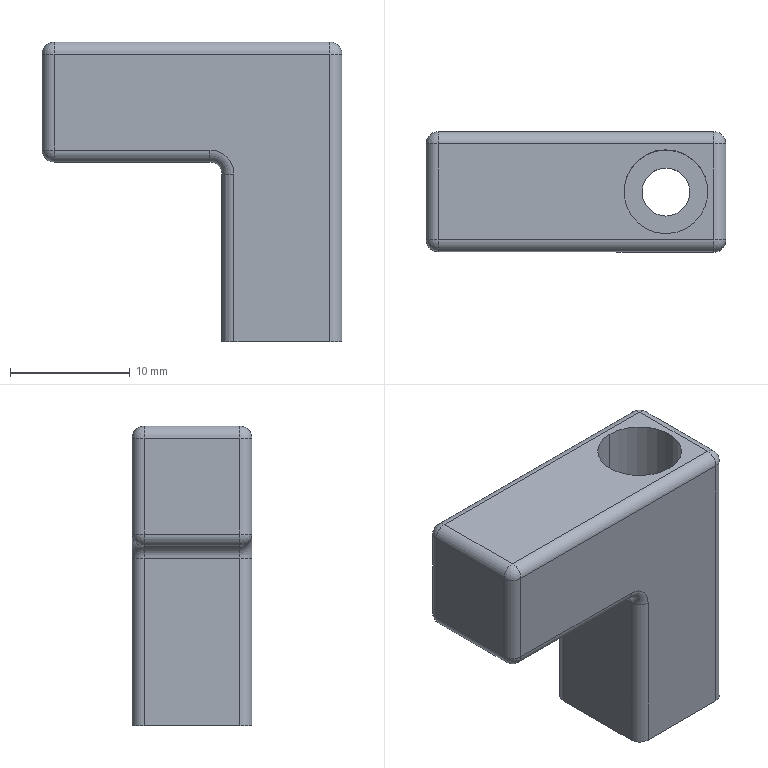NC program | NX | posted with a generic post | part box 25 x 10 x 25 mm
Lines 1 to 1607 of 2000, first 1374 of 1599 lines:
N10 G17 G21 G94 G90
(FLOOR_WALL , TOOL : D63)
N12 T01 M6
N14 G54
N16 G17 G0 G90 X-50. Y0. S6500 M3
N18 G43 Z13. H1
N20 Z3.
N22 G94 G1 Z0. F1250.
N24 X-47.
N26 X47.
N28 X50.
N30 Z3.
N32 G0 Z13.
N34 M5
(ZLEVEL_PROFILE , TOOL : D10)
N36 T09 M6
N38 G54
N40 G17 G0 G90 X2.496 Y10.099 S9500 M3
N42 G43 Z11. H9
N44 Z1.5
N46 G94 G1 X11.5 Z1.028 F1000.
N48 X12.106 Z0.996
N50 X13.737 Y9.707 Z0.908
N52 X15.2 Y8.886 Z0.821
N54 X16.386 Y7.7 Z0.733
N56 X17.206 Y6.237 Z0.645
N58 X17.599 Y4.606 Z0.557
N60 Y4. Z0.525
N62 Y-4. Z0.106
N64 Y-4.606 Z0.074
N66 X17.206 Y-6.237 Z-0.014
N68 X16.386 Y-7.7 Z-0.102
N70 X15.2 Y-8.886 Z-0.19
N72 X13.737 Y-9.707 Z-0.278
N74 X12.106 Y-10.099 Z-0.366
N76 X11.5 Z-0.397
N78 X0. Z-1.
N80 X-11.5 F3000.
N82 G2 X-17.594 Y-4.223 R6.098
N84 G1 X-17.599 Y-4.
N86 Y4.
N88 G2 X-11.5 Y10.099 R6.099
N90 G1 X11.5
N92 G2 X17.599 Y4. R6.099
N94 G1 Y-4.
N96 G2 X11.5 Y-10.099 R6.099
N98 G1 X0.
N100 X-0.387 Y-10.1 Z-1.007
N102 X-10.839 Z-1.189
N104 X-11.226 Z-1.196
N106 X-11.613 Y-10.099 Z-1.203
N108 X-11.999 Y-10.08 Z-1.209
N110 X-12.384 Y-10.036 Z-1.216
N112 X-12.765 Y-9.967 Z-1.223
N114 X-13.141 Y-9.875 Z-1.23
N116 X-13.51 Y-9.759 Z-1.236
N118 X-13.871 Y-9.62 Z-1.243
N120 X-14.223 Y-9.458 Z-1.25
N122 X-14.564 Y-9.275 Z-1.257
N124 X-14.892 Y-9.07 Z-1.264
N126 X-15.207 Y-8.844 Z-1.27
N128 X-15.507 Y-8.6 Z-1.277
N130 X-15.79 Y-8.336 Z-1.284
N132 X-16.057 Y-8.055 Z-1.291
N134 X-16.305 Y-7.758 Z-1.297
N136 X-16.533 Y-7.446 Z-1.304
N138 X-16.742 Y-7.12 Z-1.311
N140 X-16.929 Y-6.781 Z-1.318
N142 X-17.095 Y-6.431 Z-1.324
N144 X-17.238 Y-6.071 Z-1.331
N146 X-17.357 Y-5.703 Z-1.338
N148 X-17.454 Y-5.328 Z-1.345
N150 X-17.526 Y-4.948 Z-1.351
N152 X-17.574 Y-4.564 Z-1.358
N154 X-17.597 Y-4.177 Z-1.365
N156 X-17.6 Y-3.79 Z-1.372
N158 Y-3.403 Z-1.378
N160 Y3.565 Z-1.5
N162 Y3.952 Z-1.507
N164 X-17.591 Y4.339 Z-1.514
N166 X-17.557 Y4.724 Z-1.52
N168 X-17.499 Y5.107 Z-1.527
N170 X-17.416 Y5.485 Z-1.534
N172 X-17.31 Y5.857 Z-1.541
N174 X-17.181 Y6.222 Z-1.547
N176 X-17.028 Y6.578 Z-1.554
N178 X-16.854 Y6.924 Z-1.561
N180 X-16.658 Y7.257 Z-1.568
N182 X-16.441 Y7.578 Z-1.574
N184 X-16.204 Y7.884 Z-1.581
N186 X-15.948 Y8.174 Z-1.588
N188 X-15.674 Y8.448 Z-1.595
N190 X-15.384 Y8.704 Z-1.601
N192 X-15.078 Y8.941 Z-1.608
N194 X-14.757 Y9.158 Z-1.615
N196 X-14.423 Y9.354 Z-1.622
N198 X-14.078 Y9.529 Z-1.628
N200 X-13.722 Y9.681 Z-1.635
N202 X-13.357 Y9.81 Z-1.642
N204 X-12.985 Y9.916 Z-1.649
N206 X-12.607 Y9.999 Z-1.655
N208 X-12.224 Y10.057 Z-1.662
N210 X-11.838 Y10.091 Z-1.669
N212 X-11.451 Y10.1 Z-1.676
N214 X7.129 Z-2.
N216 X11.5
N218 G2 X17.6 Y4. R6.1
N220 G1 Y-4.
N222 G2 X11.5 Y-10.1 R6.1
N224 G1 X0.
N226 X-10.839 Z-2.189
N228 X-11.226 Z-2.196
N230 X-11.613 Y-10.099 Z-2.203
N232 X-11.999 Y-10.08 Z-2.209
N234 X-12.384 Y-10.036 Z-2.216
N236 X-12.765 Y-9.967 Z-2.223
N238 X-13.141 Y-9.875 Z-2.23
N240 X-13.51 Y-9.759 Z-2.236
N242 X-13.871 Y-9.62 Z-2.243
N244 X-14.223 Y-9.459 Z-2.25
N246 X-14.564 Y-9.275 Z-2.257
N248 X-14.892 Y-9.07 Z-2.264
N250 X-15.207 Y-8.845 Z-2.27
N252 X-15.506 Y-8.6 Z-2.277
N254 X-15.79 Y-8.337 Z-2.284
N256 X-16.056 Y-8.056 Z-2.291
N258 X-16.304 Y-7.759 Z-2.297
N260 X-16.533 Y-7.446 Z-2.304
N262 X-16.742 Y-7.12 Z-2.311
N264 X-16.929 Y-6.782 Z-2.318
N266 X-17.094 Y-6.432 Z-2.324
N268 X-17.237 Y-6.072 Z-2.331
N270 X-17.357 Y-5.704 Z-2.338
N272 X-17.453 Y-5.329 Z-2.345
N274 X-17.526 Y-4.949 Z-2.351
N276 X-17.574 Y-4.565 Z-2.358
N278 X-17.597 Y-4.179 Z-2.365
N280 X-17.6 Y-3.792 Z-2.372
N282 Y-3.405 Z-2.378
N284 Y3.563 Z-2.5
N286 Y3.95 Z-2.507
N288 X-17.591 Y4.337 Z-2.514
N290 X-17.557 Y4.723 Z-2.52
N292 X-17.499 Y5.105 Z-2.527
N294 X-17.417 Y5.484 Z-2.534
N296 X-17.311 Y5.856 Z-2.541
N298 X-17.181 Y6.221 Z-2.547
N300 X-17.029 Y6.576 Z-2.554
N302 X-16.855 Y6.922 Z-2.561
N304 X-16.659 Y7.256 Z-2.568
N306 X-16.442 Y7.576 Z-2.574
N308 X-16.205 Y7.882 Z-2.581
N310 X-15.949 Y8.173 Z-2.588
N312 X-15.676 Y8.447 Z-2.595
N314 X-15.385 Y8.702 Z-2.601
N316 X-15.079 Y8.939 Z-2.608
N318 X-14.759 Y9.156 Z-2.615
N320 X-14.425 Y9.353 Z-2.622
N322 X-14.08 Y9.527 Z-2.628
N324 X-13.724 Y9.68 Z-2.635
N326 X-13.36 Y9.81 Z-2.642
N328 X-12.988 Y9.916 Z-2.649
N330 X-12.609 Y9.998 Z-2.655
N332 X-12.227 Y10.057 Z-2.662
N334 X-11.841 Y10.09 Z-2.669
N336 X-11.454 Y10.1 Z-2.676
N338 X7.126 Z-3.
N340 X11.5
N342 G2 X17.6 Y4. R6.1
N344 G1 Y-4.
N346 G2 X11.5 Y-10.1 R6.1
N348 G1 X0.
N350 X-10.839 Z-3.189
N352 X-11.226 Z-3.196
N354 X-11.613 Y-10.099 Z-3.203
N356 X-11.999 Y-10.08 Z-3.209
N358 X-12.384 Y-10.036 Z-3.216
N360 X-12.765 Y-9.967 Z-3.223
N362 X-13.141 Y-9.875 Z-3.23
N364 X-13.51 Y-9.759 Z-3.236
N366 X-13.871 Y-9.62 Z-3.243
N368 X-14.223 Y-9.459 Z-3.25
N370 X-14.564 Y-9.275 Z-3.257
N372 X-14.892 Y-9.07 Z-3.264
N374 X-15.207 Y-8.845 Z-3.27
N376 X-15.506 Y-8.6 Z-3.277
N378 X-15.79 Y-8.337 Z-3.284
N380 X-16.056 Y-8.056 Z-3.291
N382 X-16.304 Y-7.759 Z-3.297
N384 X-16.533 Y-7.446 Z-3.304
N386 X-16.742 Y-7.12 Z-3.311
N388 X-16.929 Y-6.782 Z-3.318
N390 X-17.094 Y-6.432 Z-3.324
N392 X-17.237 Y-6.072 Z-3.331
N394 X-17.357 Y-5.704 Z-3.338
N396 X-17.453 Y-5.329 Z-3.345
N398 X-17.526 Y-4.949 Z-3.351
N400 X-17.574 Y-4.565 Z-3.358
N402 X-17.597 Y-4.179 Z-3.365
N404 X-17.6 Y-3.792 Z-3.372
N406 Y-3.405 Z-3.378
N408 Y3.563 Z-3.5
N410 Y3.95 Z-3.507
N412 X-17.591 Y4.337 Z-3.514
N414 X-17.557 Y4.723 Z-3.52
N416 X-17.499 Y5.105 Z-3.527
N418 X-17.417 Y5.484 Z-3.534
N420 X-17.311 Y5.856 Z-3.541
N422 X-17.181 Y6.221 Z-3.547
N424 X-17.029 Y6.576 Z-3.554
N426 X-16.855 Y6.922 Z-3.561
N428 X-16.659 Y7.256 Z-3.568
N430 X-16.442 Y7.576 Z-3.574
N432 X-16.205 Y7.882 Z-3.581
N434 X-15.949 Y8.173 Z-3.588
N436 X-15.676 Y8.447 Z-3.595
N438 X-15.385 Y8.702 Z-3.601
N440 X-15.079 Y8.939 Z-3.608
N442 X-14.759 Y9.156 Z-3.615
N444 X-14.425 Y9.353 Z-3.622
N446 X-14.08 Y9.527 Z-3.628
N448 X-13.724 Y9.68 Z-3.635
N450 X-13.36 Y9.81 Z-3.642
N452 X-12.988 Y9.916 Z-3.649
N454 X-12.609 Y9.998 Z-3.655
N456 X-12.227 Y10.057 Z-3.662
N458 X-11.841 Y10.09 Z-3.669
N460 X-11.454 Y10.1 Z-3.676
N462 X7.126 Z-4.
N464 X11.5
N466 G2 X17.6 Y4. R6.1
N468 G1 Y-4.
N470 G2 X11.5 Y-10.1 R6.1
N472 G1 X0.
N474 X-10.839 Z-4.189
N476 X-11.226 Z-4.196
N478 X-11.613 Y-10.099 Z-4.203
N480 X-11.999 Y-10.08 Z-4.209
N482 X-12.384 Y-10.036 Z-4.216
N484 X-12.765 Y-9.967 Z-4.223
N486 X-13.141 Y-9.875 Z-4.23
N488 X-13.51 Y-9.759 Z-4.236
N490 X-13.871 Y-9.62 Z-4.243
N492 X-14.223 Y-9.459 Z-4.25
N494 X-14.564 Y-9.275 Z-4.257
N496 X-14.892 Y-9.07 Z-4.264
N498 X-15.207 Y-8.845 Z-4.27
N500 X-15.506 Y-8.6 Z-4.277
N502 X-15.79 Y-8.337 Z-4.284
N504 X-16.056 Y-8.056 Z-4.291
N506 X-16.304 Y-7.759 Z-4.297
N508 X-16.533 Y-7.446 Z-4.304
N510 X-16.742 Y-7.12 Z-4.311
N512 X-16.929 Y-6.782 Z-4.318
N514 X-17.094 Y-6.432 Z-4.324
N516 X-17.237 Y-6.072 Z-4.331
N518 X-17.357 Y-5.704 Z-4.338
N520 X-17.453 Y-5.329 Z-4.345
N522 X-17.526 Y-4.949 Z-4.351
N524 X-17.574 Y-4.565 Z-4.358
N526 X-17.597 Y-4.179 Z-4.365
N528 X-17.6 Y-3.792 Z-4.372
N530 Y-3.405 Z-4.378
N532 Y3.563 Z-4.5
N534 Y3.95 Z-4.507
N536 X-17.591 Y4.337 Z-4.514
N538 X-17.557 Y4.723 Z-4.52
N540 X-17.499 Y5.105 Z-4.527
N542 X-17.417 Y5.484 Z-4.534
N544 X-17.311 Y5.856 Z-4.541
N546 X-17.181 Y6.221 Z-4.547
N548 X-17.029 Y6.576 Z-4.554
N550 X-16.855 Y6.922 Z-4.561
N552 X-16.659 Y7.256 Z-4.568
N554 X-16.442 Y7.576 Z-4.574
N556 X-16.205 Y7.882 Z-4.581
N558 X-15.949 Y8.173 Z-4.588
N560 X-15.676 Y8.447 Z-4.595
N562 X-15.385 Y8.702 Z-4.601
N564 X-15.079 Y8.939 Z-4.608
N566 X-14.759 Y9.156 Z-4.615
N568 X-14.425 Y9.353 Z-4.622
N570 X-14.08 Y9.527 Z-4.628
N572 X-13.724 Y9.68 Z-4.635
N574 X-13.36 Y9.81 Z-4.642
N576 X-12.988 Y9.916 Z-4.649
N578 X-12.609 Y9.998 Z-4.655
N580 X-12.227 Y10.057 Z-4.662
N582 X-11.841 Y10.09 Z-4.669
N584 X-11.454 Y10.1 Z-4.676
N586 X7.126 Z-5.
N588 X11.5
N590 G2 X17.6 Y4. R6.1
N592 G1 Y-4.
N594 G2 X11.5 Y-10.1 R6.1
N596 G1 X0.
N598 X-10.839 Z-5.189
N600 X-11.226 Z-5.196
N602 X-11.613 Y-10.099 Z-5.203
N604 X-11.999 Y-10.08 Z-5.209
N606 X-12.384 Y-10.036 Z-5.216
N608 X-12.765 Y-9.967 Z-5.223
N610 X-13.141 Y-9.875 Z-5.23
N612 X-13.51 Y-9.759 Z-5.236
N614 X-13.871 Y-9.62 Z-5.243
N616 X-14.223 Y-9.459 Z-5.25
N618 X-14.564 Y-9.275 Z-5.257
N620 X-14.892 Y-9.07 Z-5.264
N622 X-15.207 Y-8.845 Z-5.27
N624 X-15.506 Y-8.6 Z-5.277
N626 X-15.79 Y-8.337 Z-5.284
N628 X-16.056 Y-8.056 Z-5.291
N630 X-16.304 Y-7.759 Z-5.297
N632 X-16.533 Y-7.446 Z-5.304
N634 X-16.742 Y-7.12 Z-5.311
N636 X-16.929 Y-6.782 Z-5.318
N638 X-17.094 Y-6.432 Z-5.324
N640 X-17.237 Y-6.072 Z-5.331
N642 X-17.357 Y-5.704 Z-5.338
N644 X-17.453 Y-5.329 Z-5.345
N646 X-17.526 Y-4.949 Z-5.351
N648 X-17.574 Y-4.565 Z-5.358
N650 X-17.597 Y-4.179 Z-5.365
N652 X-17.6 Y-3.792 Z-5.372
N654 Y-3.405 Z-5.378
N656 Y3.563 Z-5.5
N658 Y3.95 Z-5.507
N660 X-17.591 Y4.337 Z-5.514
N662 X-17.557 Y4.723 Z-5.52
N664 X-17.499 Y5.105 Z-5.527
N666 X-17.417 Y5.484 Z-5.534
N668 X-17.311 Y5.856 Z-5.541
N670 X-17.181 Y6.221 Z-5.547
N672 X-17.029 Y6.576 Z-5.554
N674 X-16.855 Y6.922 Z-5.561
N676 X-16.659 Y7.256 Z-5.568
N678 X-16.442 Y7.576 Z-5.574
N680 X-16.205 Y7.882 Z-5.581
N682 X-15.949 Y8.173 Z-5.588
N684 X-15.676 Y8.447 Z-5.595
N686 X-15.385 Y8.702 Z-5.601
N688 X-15.079 Y8.939 Z-5.608
N690 X-14.759 Y9.156 Z-5.615
N692 X-14.425 Y9.353 Z-5.622
N694 X-14.08 Y9.527 Z-5.628
N696 X-13.724 Y9.68 Z-5.635
N698 X-13.36 Y9.81 Z-5.642
N700 X-12.988 Y9.916 Z-5.649
N702 X-12.609 Y9.998 Z-5.655
N704 X-12.227 Y10.057 Z-5.662
N706 X-11.841 Y10.09 Z-5.669
N708 X-11.454 Y10.1 Z-5.676
N710 X7.126 Z-6.
N712 X11.5
N714 G2 X17.6 Y4. R6.1
N716 G1 Y-4.
N718 G2 X11.5 Y-10.1 R6.1
N720 G1 X0.
N722 X-10.839 Z-6.189
N724 X-11.226 Z-6.196
N726 X-11.613 Y-10.099 Z-6.203
N728 X-11.999 Y-10.08 Z-6.209
N730 X-12.384 Y-10.036 Z-6.216
N732 X-12.765 Y-9.967 Z-6.223
N734 X-13.141 Y-9.875 Z-6.23
N736 X-13.51 Y-9.759 Z-6.236
N738 X-13.871 Y-9.62 Z-6.243
N740 X-14.223 Y-9.459 Z-6.25
N742 X-14.564 Y-9.275 Z-6.257
N744 X-14.892 Y-9.07 Z-6.264
N746 X-15.207 Y-8.845 Z-6.27
N748 X-15.506 Y-8.6 Z-6.277
N750 X-15.79 Y-8.337 Z-6.284
N752 X-16.056 Y-8.056 Z-6.291
N754 X-16.304 Y-7.759 Z-6.297
N756 X-16.533 Y-7.446 Z-6.304
N758 X-16.742 Y-7.12 Z-6.311
N760 X-16.929 Y-6.782 Z-6.318
N762 X-17.094 Y-6.432 Z-6.324
N764 X-17.237 Y-6.072 Z-6.331
N766 X-17.357 Y-5.704 Z-6.338
N768 X-17.453 Y-5.329 Z-6.345
N770 X-17.526 Y-4.949 Z-6.351
N772 X-17.574 Y-4.565 Z-6.358
N774 X-17.597 Y-4.179 Z-6.365
N776 X-17.6 Y-3.792 Z-6.372
N778 Y-3.405 Z-6.378
N780 Y3.563 Z-6.5
N782 Y3.95 Z-6.507
N784 X-17.591 Y4.337 Z-6.514
N786 X-17.557 Y4.723 Z-6.52
N788 X-17.499 Y5.105 Z-6.527
N790 X-17.417 Y5.484 Z-6.534
N792 X-17.311 Y5.856 Z-6.541
N794 X-17.181 Y6.221 Z-6.547
N796 X-17.029 Y6.576 Z-6.554
N798 X-16.855 Y6.922 Z-6.561
N800 X-16.659 Y7.256 Z-6.568
N802 X-16.442 Y7.576 Z-6.574
N804 X-16.205 Y7.882 Z-6.581
N806 X-15.949 Y8.173 Z-6.588
N808 X-15.676 Y8.447 Z-6.595
N810 X-15.385 Y8.702 Z-6.601
N812 X-15.079 Y8.939 Z-6.608
N814 X-14.759 Y9.156 Z-6.615
N816 X-14.425 Y9.353 Z-6.622
N818 X-14.08 Y9.527 Z-6.628
N820 X-13.724 Y9.68 Z-6.635
N822 X-13.36 Y9.81 Z-6.642
N824 X-12.988 Y9.916 Z-6.649
N826 X-12.609 Y9.998 Z-6.655
N828 X-12.227 Y10.057 Z-6.662
N830 X-11.841 Y10.09 Z-6.669
N832 X-11.454 Y10.1 Z-6.676
N834 X7.126 Z-7.
N836 X11.5
N838 G2 X17.6 Y4. R6.1
N840 G1 Y-4.
N842 G2 X11.5 Y-10.1 R6.1
N844 G1 X0.
N846 X-10.839 Z-7.189
N848 X-11.226 Z-7.196
N850 X-11.613 Y-10.099 Z-7.203
N852 X-11.999 Y-10.08 Z-7.209
N854 X-12.384 Y-10.036 Z-7.216
N856 X-12.765 Y-9.967 Z-7.223
N858 X-13.141 Y-9.875 Z-7.23
N860 X-13.51 Y-9.759 Z-7.236
N862 X-13.871 Y-9.62 Z-7.243
N864 X-14.223 Y-9.459 Z-7.25
N866 X-14.564 Y-9.275 Z-7.257
N868 X-14.892 Y-9.07 Z-7.264
N870 X-15.207 Y-8.845 Z-7.27
N872 X-15.506 Y-8.6 Z-7.277
N874 X-15.79 Y-8.337 Z-7.284
N876 X-16.056 Y-8.056 Z-7.291
N878 X-16.304 Y-7.759 Z-7.297
N880 X-16.533 Y-7.446 Z-7.304
N882 X-16.742 Y-7.12 Z-7.311
N884 X-16.929 Y-6.782 Z-7.318
N886 X-17.094 Y-6.432 Z-7.324
N888 X-17.237 Y-6.072 Z-7.331
N890 X-17.357 Y-5.704 Z-7.338
N892 X-17.453 Y-5.329 Z-7.345
N894 X-17.526 Y-4.949 Z-7.351
N896 X-17.574 Y-4.565 Z-7.358
N898 X-17.597 Y-4.179 Z-7.365
N900 X-17.6 Y-3.792 Z-7.372
N902 Y-3.405 Z-7.378
N904 Y3.563 Z-7.5
N906 Y3.95 Z-7.507
N908 X-17.591 Y4.337 Z-7.514
N910 X-17.557 Y4.723 Z-7.52
N912 X-17.499 Y5.105 Z-7.527
N914 X-17.417 Y5.484 Z-7.534
N916 X-17.311 Y5.856 Z-7.541
N918 X-17.181 Y6.221 Z-7.547
N920 X-17.029 Y6.576 Z-7.554
N922 X-16.855 Y6.922 Z-7.561
N924 X-16.659 Y7.256 Z-7.568
N926 X-16.442 Y7.576 Z-7.574
N928 X-16.205 Y7.882 Z-7.581
N930 X-15.949 Y8.173 Z-7.588
N932 X-15.676 Y8.447 Z-7.595
N934 X-15.385 Y8.702 Z-7.601
N936 X-15.079 Y8.939 Z-7.608
N938 X-14.759 Y9.156 Z-7.615
N940 X-14.425 Y9.353 Z-7.622
N942 X-14.08 Y9.527 Z-7.628
N944 X-13.724 Y9.68 Z-7.635
N946 X-13.36 Y9.81 Z-7.642
N948 X-12.988 Y9.916 Z-7.649
N950 X-12.609 Y9.998 Z-7.655
N952 X-12.227 Y10.057 Z-7.662
N954 X-11.841 Y10.09 Z-7.669
N956 X-11.454 Y10.1 Z-7.676
N958 X7.126 Z-8.
N960 X11.5
N962 G2 X17.6 Y4. R6.1
N964 G1 Y-4.
N966 G2 X11.5 Y-10.1 R6.1
N968 G1 X0.
N970 X-10.839 Z-8.189
N972 X-11.226 Z-8.196
N974 X-11.613 Y-10.099 Z-8.203
N976 X-11.999 Y-10.08 Z-8.209
N978 X-12.384 Y-10.036 Z-8.216
N980 X-12.765 Y-9.967 Z-8.223
N982 X-13.141 Y-9.875 Z-8.23
N984 X-13.51 Y-9.759 Z-8.236
N986 X-13.871 Y-9.62 Z-8.243
N988 X-14.223 Y-9.459 Z-8.25
N990 X-14.564 Y-9.275 Z-8.257
N992 X-14.892 Y-9.07 Z-8.264
N994 X-15.207 Y-8.845 Z-8.27
N996 X-15.506 Y-8.6 Z-8.277
N998 X-15.79 Y-8.337 Z-8.284
N1000 X-16.056 Y-8.056 Z-8.291
N1002 X-16.304 Y-7.759 Z-8.297
N1004 X-16.533 Y-7.446 Z-8.304
N1006 X-16.742 Y-7.12 Z-8.311
N1008 X-16.929 Y-6.782 Z-8.318
N1010 X-17.094 Y-6.432 Z-8.324
N1012 X-17.237 Y-6.072 Z-8.331
N1014 X-17.357 Y-5.704 Z-8.338
N1016 X-17.453 Y-5.329 Z-8.345
N1018 X-17.526 Y-4.949 Z-8.351
N1020 X-17.574 Y-4.565 Z-8.358
N1022 X-17.597 Y-4.179 Z-8.365
N1024 X-17.6 Y-3.792 Z-8.372
N1026 Y-3.405 Z-8.378
N1028 Y3.563 Z-8.5
N1030 Y3.95 Z-8.507
N1032 X-17.591 Y4.337 Z-8.514
N1034 X-17.557 Y4.723 Z-8.52
N1036 X-17.499 Y5.105 Z-8.527
N1038 X-17.417 Y5.484 Z-8.534
N1040 X-17.311 Y5.856 Z-8.541
N1042 X-17.181 Y6.221 Z-8.547
N1044 X-17.029 Y6.576 Z-8.554
N1046 X-16.855 Y6.922 Z-8.561
N1048 X-16.659 Y7.256 Z-8.568
N1050 X-16.442 Y7.576 Z-8.574
N1052 X-16.205 Y7.882 Z-8.581
N1054 X-15.949 Y8.173 Z-8.588
N1056 X-15.676 Y8.447 Z-8.595
N1058 X-15.385 Y8.702 Z-8.601
N1060 X-15.079 Y8.939 Z-8.608
N1062 X-14.759 Y9.156 Z-8.615
N1064 X-14.425 Y9.353 Z-8.622
N1066 X-14.08 Y9.527 Z-8.628
N1068 X-13.724 Y9.68 Z-8.635
N1070 X-13.36 Y9.81 Z-8.642
N1072 X-12.988 Y9.916 Z-8.649
N1074 X-12.609 Y9.998 Z-8.655
N1076 X-12.227 Y10.057 Z-8.662
N1078 X-11.841 Y10.09 Z-8.669
N1080 X-11.454 Y10.1 Z-8.676
N1082 X7.126 Z-9.
N1084 X11.5
N1086 G2 X17.6 Y4. R6.1
N1088 G1 Y-4.
N1090 G2 X11.5 Y-10.1 R6.1
N1092 G1 X0.
N1094 X-10.839 Z-9.189
N1096 X-11.226 Z-9.196
N1098 X-11.613 Y-10.099 Z-9.203
N1100 X-11.999 Y-10.08 Z-9.209
N1102 X-12.384 Y-10.036 Z-9.216
N1104 X-12.765 Y-9.967 Z-9.223
N1106 X-13.141 Y-9.875 Z-9.23
N1108 X-13.51 Y-9.759 Z-9.236
N1110 X-13.871 Y-9.62 Z-9.243
N1112 X-14.223 Y-9.459 Z-9.25
N1114 X-14.564 Y-9.275 Z-9.257
N1116 X-14.892 Y-9.07 Z-9.264
N1118 X-15.207 Y-8.845 Z-9.27
N1120 X-15.506 Y-8.6 Z-9.277
N1122 X-15.79 Y-8.337 Z-9.284
N1124 X-16.056 Y-8.056 Z-9.291
N1126 X-16.304 Y-7.759 Z-9.297
N1128 X-16.533 Y-7.446 Z-9.304
N1130 X-16.742 Y-7.12 Z-9.311
N1132 X-16.929 Y-6.782 Z-9.318
N1134 X-17.094 Y-6.432 Z-9.324
N1136 X-17.237 Y-6.072 Z-9.331
N1138 X-17.357 Y-5.704 Z-9.338
N1140 X-17.453 Y-5.329 Z-9.345
N1142 X-17.526 Y-4.949 Z-9.351
N1144 X-17.574 Y-4.565 Z-9.358
N1146 X-17.597 Y-4.179 Z-9.365
N1148 X-17.6 Y-3.792 Z-9.372
N1150 Y-3.405 Z-9.378
N1152 Y3.563 Z-9.5
N1154 Y3.95 Z-9.507
N1156 X-17.591 Y4.337 Z-9.514
N1158 X-17.557 Y4.723 Z-9.52
N1160 X-17.499 Y5.105 Z-9.527
N1162 X-17.417 Y5.484 Z-9.534
N1164 X-17.311 Y5.856 Z-9.541
N1166 X-17.181 Y6.221 Z-9.547
N1168 X-17.029 Y6.576 Z-9.554
N1170 X-16.855 Y6.922 Z-9.561
N1172 X-16.659 Y7.256 Z-9.568
N1174 X-16.442 Y7.576 Z-9.574
N1176 X-16.205 Y7.882 Z-9.581
N1178 X-15.949 Y8.173 Z-9.588
N1180 X-15.676 Y8.447 Z-9.595
N1182 X-15.385 Y8.702 Z-9.601
N1184 X-15.079 Y8.939 Z-9.608
N1186 X-14.759 Y9.156 Z-9.615
N1188 X-14.425 Y9.353 Z-9.622
N1190 X-14.08 Y9.527 Z-9.628
N1192 X-13.724 Y9.68 Z-9.635
N1194 X-13.36 Y9.81 Z-9.642
N1196 X-12.988 Y9.916 Z-9.649
N1198 X-12.609 Y9.998 Z-9.655
N1200 X-12.227 Y10.057 Z-9.662
N1202 X-11.841 Y10.09 Z-9.669
N1204 X-11.454 Y10.1 Z-9.676
N1206 X7.126 Z-10.
N1208 X11.5
N1210 G2 X17.6 Y4. R6.1
N1212 G1 Y-4.
N1214 G2 X11.5 Y-10.1 R6.1
N1216 G1 X0.
N1218 X-10.839 Z-10.189
N1220 X-11.226 Z-10.196
N1222 X-11.613 Y-10.099 Z-10.203
N1224 X-11.999 Y-10.08 Z-10.209
N1226 X-12.384 Y-10.036 Z-10.216
N1228 X-12.765 Y-9.967 Z-10.223
N1230 X-13.141 Y-9.875 Z-10.23
N1232 X-13.51 Y-9.759 Z-10.236
N1234 X-13.871 Y-9.62 Z-10.243
N1236 X-14.223 Y-9.459 Z-10.25
N1238 X-14.564 Y-9.275 Z-10.257
N1240 X-14.892 Y-9.07 Z-10.264
N1242 X-15.207 Y-8.845 Z-10.27
N1244 X-15.506 Y-8.6 Z-10.277
N1246 X-15.79 Y-8.337 Z-10.284
N1248 X-16.056 Y-8.056 Z-10.291
N1250 X-16.304 Y-7.759 Z-10.297
N1252 X-16.533 Y-7.446 Z-10.304
N1254 X-16.742 Y-7.12 Z-10.311
N1256 X-16.929 Y-6.782 Z-10.318
N1258 X-17.094 Y-6.432 Z-10.324
N1260 X-17.237 Y-6.072 Z-10.331
N1262 X-17.357 Y-5.704 Z-10.338
N1264 X-17.453 Y-5.329 Z-10.345
N1266 X-17.526 Y-4.949 Z-10.351
N1268 X-17.574 Y-4.565 Z-10.358
N1270 X-17.597 Y-4.179 Z-10.365
N1272 X-17.6 Y-3.792 Z-10.372
N1274 Y-3.405 Z-10.378
N1276 Y3.563 Z-10.5
N1278 Y3.95 Z-10.507
N1280 X-17.591 Y4.337 Z-10.514
N1282 X-17.557 Y4.723 Z-10.52
N1284 X-17.499 Y5.105 Z-10.527
N1286 X-17.417 Y5.484 Z-10.534
N1288 X-17.311 Y5.856 Z-10.541
N1290 X-17.181 Y6.221 Z-10.547
N1292 X-17.029 Y6.576 Z-10.554
N1294 X-16.855 Y6.922 Z-10.561
N1296 X-16.659 Y7.256 Z-10.568
N1298 X-16.442 Y7.576 Z-10.574
N1300 X-16.205 Y7.882 Z-10.581
N1302 X-15.949 Y8.173 Z-10.588
N1304 X-15.676 Y8.447 Z-10.595
N1306 X-15.385 Y8.702 Z-10.601
N1308 X-15.079 Y8.939 Z-10.608
N1310 X-14.759 Y9.156 Z-10.615
N1312 X-14.425 Y9.353 Z-10.622
N1314 X-14.08 Y9.527 Z-10.628
N1316 X-13.724 Y9.68 Z-10.635
N1318 X-13.36 Y9.81 Z-10.642
N1320 X-12.988 Y9.916 Z-10.649
N1322 X-12.609 Y9.998 Z-10.655
N1324 X-12.227 Y10.057 Z-10.662
N1326 X-11.841 Y10.09 Z-10.669
N1328 X-11.454 Y10.1 Z-10.676
N1330 X7.126 Z-11.
N1332 X11.5
N1334 G2 X17.6 Y4. R6.1
N1336 G1 Y-4.
N1338 G2 X11.5 Y-10.1 R6.1
N1340 G1 X0.
N1342 X-10.839 Z-11.189
N1344 X-11.226 Z-11.196
N1346 X-11.613 Y-10.099 Z-11.203
N1348 X-11.999 Y-10.08 Z-11.209
N1350 X-12.384 Y-10.036 Z-11.216
N1352 X-12.765 Y-9.967 Z-11.223
N1354 X-13.141 Y-9.875 Z-11.23
N1356 X-13.51 Y-9.759 Z-11.236
N1358 X-13.871 Y-9.62 Z-11.243
N1360 X-14.223 Y-9.459 Z-11.25
N1362 X-14.564 Y-9.275 Z-11.257
N1364 X-14.892 Y-9.07 Z-11.264
N1366 X-15.207 Y-8.845 Z-11.27
N1368 X-15.506 Y-8.6 Z-11.277
N1370 X-15.79 Y-8.337 Z-11.284
N1372 X-16.056 Y-8.056 Z-11.291
N1374 X-16.304 Y-7.759 Z-11.297
N1376 X-16.533 Y-7.446 Z-11.304
N1378 X-16.742 Y-7.12 Z-11.311
N1380 X-16.929 Y-6.782 Z-11.318
N1382 X-17.094 Y-6.432 Z-11.324
N1384 X-17.237 Y-6.072 Z-11.331
N1386 X-17.357 Y-5.704 Z-11.338
N1388 X-17.453 Y-5.329 Z-11.345
N1390 X-17.526 Y-4.949 Z-11.351
N1392 X-17.574 Y-4.565 Z-11.358
N1394 X-17.597 Y-4.179 Z-11.365
N1396 X-17.6 Y-3.792 Z-11.372
N1398 Y-3.405 Z-11.378
N1400 Y3.563 Z-11.5
N1402 Y3.95 Z-11.507
N1404 X-17.591 Y4.337 Z-11.514
N1406 X-17.557 Y4.723 Z-11.52
N1408 X-17.499 Y5.105 Z-11.527
N1410 X-17.417 Y5.484 Z-11.534
N1412 X-17.311 Y5.856 Z-11.541
N1414 X-17.181 Y6.221 Z-11.547
N1416 X-17.029 Y6.576 Z-11.554
N1418 X-16.855 Y6.922 Z-11.561
N1420 X-16.659 Y7.256 Z-11.568
N1422 X-16.442 Y7.576 Z-11.574
N1424 X-16.205 Y7.882 Z-11.581
N1426 X-15.949 Y8.173 Z-11.588
N1428 X-15.676 Y8.447 Z-11.595
N1430 X-15.385 Y8.702 Z-11.601
N1432 X-15.079 Y8.939 Z-11.608
N1434 X-14.759 Y9.156 Z-11.615
N1436 X-14.425 Y9.353 Z-11.622
N1438 X-14.08 Y9.527 Z-11.628
N1440 X-13.724 Y9.68 Z-11.635
N1442 X-13.36 Y9.81 Z-11.642
N1444 X-12.988 Y9.916 Z-11.649
N1446 X-12.609 Y9.998 Z-11.655
N1448 X-12.227 Y10.057 Z-11.662
N1450 X-11.841 Y10.09 Z-11.669
N1452 X-11.454 Y10.1 Z-11.676
N1454 X7.126 Z-12.
N1456 X11.5
N1458 G2 X17.6 Y4. R6.1
N1460 G1 Y-4.
N1462 G2 X11.5 Y-10.1 R6.1
N1464 G1 X0.
N1466 X-10.839 Z-12.189
N1468 X-11.226 Z-12.196
N1470 X-11.613 Y-10.099 Z-12.203
N1472 X-11.999 Y-10.08 Z-12.209
N1474 X-12.384 Y-10.036 Z-12.216
N1476 X-12.765 Y-9.967 Z-12.223
N1478 X-13.141 Y-9.875 Z-12.23
N1480 X-13.51 Y-9.759 Z-12.236
N1482 X-13.871 Y-9.62 Z-12.243
N1484 X-14.223 Y-9.459 Z-12.25
N1486 X-14.564 Y-9.275 Z-12.257
N1488 X-14.892 Y-9.07 Z-12.264
N1490 X-15.207 Y-8.845 Z-12.27
N1492 X-15.506 Y-8.6 Z-12.277
N1494 X-15.79 Y-8.337 Z-12.284
N1496 X-16.056 Y-8.056 Z-12.291
N1498 X-16.304 Y-7.759 Z-12.297
N1500 X-16.533 Y-7.446 Z-12.304
N1502 X-16.742 Y-7.12 Z-12.311
N1504 X-16.929 Y-6.782 Z-12.318
N1506 X-17.094 Y-6.432 Z-12.324
N1508 X-17.237 Y-6.072 Z-12.331
N1510 X-17.357 Y-5.704 Z-12.338
N1512 X-17.453 Y-5.329 Z-12.345
N1514 X-17.526 Y-4.949 Z-12.351
N1516 X-17.574 Y-4.565 Z-12.358
N1518 X-17.597 Y-4.179 Z-12.365
N1520 X-17.6 Y-3.792 Z-12.372
N1522 Y-3.405 Z-12.378
N1524 Y3.563 Z-12.5
N1526 Y3.95 Z-12.507
N1528 X-17.591 Y4.337 Z-12.514
N1530 X-17.557 Y4.723 Z-12.52
N1532 X-17.499 Y5.105 Z-12.527
N1534 X-17.417 Y5.484 Z-12.534
N1536 X-17.311 Y5.856 Z-12.541
N1538 X-17.181 Y6.221 Z-12.547
N1540 X-17.029 Y6.576 Z-12.554
N1542 X-16.855 Y6.922 Z-12.561
N1544 X-16.659 Y7.256 Z-12.568
N1546 X-16.442 Y7.576 Z-12.574
N1548 X-16.205 Y7.882 Z-12.581
N1550 X-15.949 Y8.173 Z-12.588
N1552 X-15.676 Y8.447 Z-12.595
N1554 X-15.385 Y8.702 Z-12.601
N1556 X-15.079 Y8.939 Z-12.608
N1558 X-14.759 Y9.156 Z-12.615
N1560 X-14.425 Y9.353 Z-12.622
N1562 X-14.08 Y9.527 Z-12.628
N1564 X-13.724 Y9.68 Z-12.635
N1566 X-13.36 Y9.81 Z-12.642
N1568 X-12.988 Y9.916 Z-12.649
N1570 X-12.609 Y9.998 Z-12.655
N1572 X-12.227 Y10.057 Z-12.662
N1574 X-11.841 Y10.09 Z-12.669
N1576 X-11.454 Y10.1 Z-12.676
N1578 X7.126 Z-13.
N1580 X11.5
N1582 G2 X17.6 Y4. R6.1
N1584 G1 Y-4.
N1586 G2 X11.5 Y-10.1 R6.1
N1588 G1 X0.
N1590 X-10.839 Z-13.189
N1592 X-11.226 Z-13.196
N1594 X-11.613 Y-10.099 Z-13.203
N1596 X-11.999 Y-10.08 Z-13.209
N1598 X-12.384 Y-10.036 Z-13.216
N1600 X-12.765 Y-9.967 Z-13.223
N1602 X-13.141 Y-9.875 Z-13.23
N1604 X-13.51 Y-9.759 Z-13.236
N1606 X-13.871 Y-9.62 Z-13.243
N1608 X-14.223 Y-9.459 Z-13.25
N1610 X-14.564 Y-9.275 Z-13.257
N1612 X-14.892 Y-9.07 Z-13.264
N1614 X-15.207 Y-8.845 Z-13.27
N1616 X-15.506 Y-8.6 Z-13.277
N1618 X-15.79 Y-8.337 Z-13.284
N1620 X-16.056 Y-8.056 Z-13.291
N1622 X-16.304 Y-7.759 Z-13.297
N1624 X-16.533 Y-7.446 Z-13.304
N1626 X-16.742 Y-7.12 Z-13.311
N1628 X-16.929 Y-6.782 Z-13.318
N1630 X-17.094 Y-6.432 Z-13.324
N1632 X-17.237 Y-6.072 Z-13.331
N1634 X-17.357 Y-5.704 Z-13.338
N1636 X-17.453 Y-5.329 Z-13.345
N1638 X-17.526 Y-4.949 Z-13.351
N1640 X-17.574 Y-4.565 Z-13.358
N1642 X-17.597 Y-4.179 Z-13.365
N1644 X-17.6 Y-3.792 Z-13.372
N1646 Y-3.405 Z-13.378
N1648 Y3.563 Z-13.5
N1650 Y3.95 Z-13.507
N1652 X-17.591 Y4.337 Z-13.514
N1654 X-17.557 Y4.723 Z-13.52
N1656 X-17.499 Y5.105 Z-13.527
N1658 X-17.417 Y5.484 Z-13.534
N1660 X-17.311 Y5.856 Z-13.541
N1662 X-17.181 Y6.221 Z-13.547
N1664 X-17.029 Y6.576 Z-13.554
N1666 X-16.855 Y6.922 Z-13.561
N1668 X-16.659 Y7.256 Z-13.568
N1670 X-16.442 Y7.576 Z-13.574
N1672 X-16.205 Y7.882 Z-13.581
N1674 X-15.949 Y8.173 Z-13.588
N1676 X-15.676 Y8.447 Z-13.595
N1678 X-15.385 Y8.702 Z-13.601
N1680 X-15.079 Y8.939 Z-13.608
N1682 X-14.759 Y9.156 Z-13.615
N1684 X-14.425 Y9.353 Z-13.622
N1686 X-14.08 Y9.527 Z-13.628
N1688 X-13.724 Y9.68 Z-13.635
N1690 X-13.36 Y9.81 Z-13.642
N1692 X-12.988 Y9.916 Z-13.649
N1694 X-12.609 Y9.998 Z-13.655
N1696 X-12.227 Y10.057 Z-13.662
N1698 X-11.841 Y10.09 Z-13.669
N1700 X-11.454 Y10.1 Z-13.676
N1702 X7.126 Z-14.
N1704 X11.5
N1706 G2 X17.6 Y4. R6.1
N1708 G1 Y-4.
N1710 G2 X11.5 Y-10.1 R6.1
N1712 G1 X0.
N1714 X-10.839 Z-14.189
N1716 X-11.226 Z-14.196
N1718 X-11.613 Y-10.099 Z-14.203
N1720 X-11.999 Y-10.08 Z-14.209
N1722 X-12.384 Y-10.036 Z-14.216
N1724 X-12.765 Y-9.967 Z-14.223
N1726 X-13.141 Y-9.875 Z-14.23
N1728 X-13.51 Y-9.759 Z-14.236
N1730 X-13.871 Y-9.62 Z-14.243
N1732 X-14.223 Y-9.459 Z-14.25
N1734 X-14.564 Y-9.275 Z-14.257
N1736 X-14.892 Y-9.07 Z-14.264
N1738 X-15.207 Y-8.845 Z-14.27
N1740 X-15.506 Y-8.6 Z-14.277
N1742 X-15.79 Y-8.337 Z-14.284
N1744 X-16.056 Y-8.056 Z-14.291
N1746 X-16.304 Y-7.759 Z-14.297
N1748 X-16.533 Y-7.446 Z-14.304
N1750 X-16.742 Y-7.12 Z-14.311
N1752 X-16.929 Y-6.782 Z-14.318
N1754 X-17.094 Y-6.432 Z-14.324
N1756 X-17.237 Y-6.072 Z-14.331
N1758 X-17.357 Y-5.704 Z-14.338
N1760 X-17.453 Y-5.329 Z-14.345
N1762 X-17.526 Y-4.949 Z-14.351
N1764 X-17.574 Y-4.565 Z-14.358
N1766 X-17.597 Y-4.179 Z-14.365
N1768 X-17.6 Y-3.792 Z-14.372
N1770 Y-3.405 Z-14.378
N1772 Y3.563 Z-14.5
N1774 Y3.95 Z-14.507
N1776 X-17.591 Y4.337 Z-14.514
N1778 X-17.557 Y4.723 Z-14.52
N1780 X-17.499 Y5.105 Z-14.527
N1782 X-17.417 Y5.484 Z-14.534
N1784 X-17.311 Y5.856 Z-14.541
N1786 X-17.181 Y6.221 Z-14.547
N1788 X-17.029 Y6.576 Z-14.554
N1790 X-16.855 Y6.922 Z-14.561
N1792 X-16.659 Y7.256 Z-14.568
N1794 X-16.442 Y7.576 Z-14.574
N1796 X-16.205 Y7.882 Z-14.581
N1798 X-15.949 Y8.173 Z-14.588
N1800 X-15.676 Y8.447 Z-14.595
N1802 X-15.385 Y8.702 Z-14.601
N1804 X-15.079 Y8.939 Z-14.608
N1806 X-14.759 Y9.156 Z-14.615
N1808 X-14.425 Y9.353 Z-14.622
N1810 X-14.08 Y9.527 Z-14.628
N1812 X-13.724 Y9.68 Z-14.635
N1814 X-13.36 Y9.81 Z-14.642
N1816 X-12.988 Y9.916 Z-14.649
N1818 X-12.609 Y9.998 Z-14.655
N1820 X-12.227 Y10.057 Z-14.662
N1822 X-11.841 Y10.09 Z-14.669
N1824 X-11.454 Y10.1 Z-14.676
N1826 X7.126 Z-15.
N1828 X11.5
N1830 G2 X17.6 Y4. R6.1
N1832 G1 Y-4.
N1834 G2 X11.5 Y-10.1 R6.1
N1836 G1 X0.
N1838 X-10.839 Z-15.189
N1840 X-11.226 Z-15.196
N1842 X-11.613 Y-10.099 Z-15.203
N1844 X-11.999 Y-10.08 Z-15.209
N1846 X-12.384 Y-10.036 Z-15.216
N1848 X-12.765 Y-9.967 Z-15.223
N1850 X-13.141 Y-9.875 Z-15.23
N1852 X-13.51 Y-9.759 Z-15.236
N1854 X-13.871 Y-9.62 Z-15.243
N1856 X-14.223 Y-9.459 Z-15.25
N1858 X-14.564 Y-9.275 Z-15.257
N1860 X-14.892 Y-9.07 Z-15.264
N1862 X-15.207 Y-8.845 Z-15.27
N1864 X-15.506 Y-8.6 Z-15.277
N1866 X-15.79 Y-8.337 Z-15.284
N1868 X-16.056 Y-8.056 Z-15.291
N1870 X-16.304 Y-7.759 Z-15.297
N1872 X-16.533 Y-7.446 Z-15.304
N1874 X-16.742 Y-7.12 Z-15.311
N1876 X-16.929 Y-6.782 Z-15.318
N1878 X-17.094 Y-6.432 Z-15.324
N1880 X-17.237 Y-6.072 Z-15.331
N1882 X-17.357 Y-5.704 Z-15.338
N1884 X-17.453 Y-5.329 Z-15.345
N1886 X-17.526 Y-4.949 Z-15.351
N1888 X-17.574 Y-4.565 Z-15.358
N1890 X-17.597 Y-4.179 Z-15.365
N1892 X-17.6 Y-3.792 Z-15.372
N1894 Y-3.405 Z-15.378
N1896 Y3.563 Z-15.5
N1898 Y3.95 Z-15.507
N1900 X-17.591 Y4.337 Z-15.514
N1902 X-17.557 Y4.723 Z-15.52
N1904 X-17.499 Y5.105 Z-15.527
N1906 X-17.417 Y5.484 Z-15.534
N1908 X-17.311 Y5.856 Z-15.541
N1910 X-17.181 Y6.221 Z-15.547
N1912 X-17.029 Y6.576 Z-15.554
N1914 X-16.855 Y6.922 Z-15.561
N1916 X-16.659 Y7.256 Z-15.568
N1918 X-16.442 Y7.576 Z-15.574
N1920 X-16.205 Y7.882 Z-15.581
N1922 X-15.949 Y8.173 Z-15.588
N1924 X-15.676 Y8.447 Z-15.595
N1926 X-15.385 Y8.702 Z-15.601
N1928 X-15.079 Y8.939 Z-15.608
N1930 X-14.759 Y9.156 Z-15.615
N1932 X-14.425 Y9.353 Z-15.622
N1934 X-14.08 Y9.527 Z-15.628
N1936 X-13.724 Y9.68 Z-15.635
N1938 X-13.36 Y9.81 Z-15.642
N1940 X-12.988 Y9.916 Z-15.649
N1942 X-12.609 Y9.998 Z-15.655
N1944 X-12.227 Y10.057 Z-15.662
N1946 X-11.841 Y10.09 Z-15.669
N1948 X-11.454 Y10.1 Z-15.676
N1950 X7.126 Z-16.
N1952 X11.5
N1954 G2 X17.6 Y4. R6.1
N1956 G1 Y-4.
N1958 G2 X11.5 Y-10.1 R6.1
N1960 G1 X0.
N1962 X-10.839 Z-16.189
N1964 X-11.226 Z-16.196
N1966 X-11.613 Y-10.099 Z-16.203
N1968 X-11.999 Y-10.08 Z-16.209
N1970 X-12.384 Y-10.036 Z-16.216
N1972 X-12.765 Y-9.967 Z-16.223
N1974 X-13.141 Y-9.875 Z-16.23
N1976 X-13.51 Y-9.759 Z-16.236
N1978 X-13.871 Y-9.62 Z-16.243
N1980 X-14.223 Y-9.459 Z-16.25
N1982 X-14.564 Y-9.275 Z-16.257
N1984 X-14.892 Y-9.07 Z-16.264
N1986 X-15.207 Y-8.845 Z-16.27
N1988 X-15.506 Y-8.6 Z-16.277
N1990 X-15.79 Y-8.337 Z-16.284
N1992 X-16.056 Y-8.056 Z-16.291
N1994 X-16.304 Y-7.759 Z-16.297
N1996 X-16.533 Y-7.446 Z-16.304
N1998 X-16.742 Y-7.12 Z-16.311
N2000 X-16.929 Y-6.782 Z-16.318
N2002 X-17.094 Y-6.432 Z-16.324
N2004 X-17.237 Y-6.072 Z-16.331
N2006 X-17.357 Y-5.704 Z-16.338
N2008 X-17.453 Y-5.329 Z-16.345
N2010 X-17.526 Y-4.949 Z-16.351
N2012 X-17.574 Y-4.565 Z-16.358
N2014 X-17.597 Y-4.179 Z-16.365
N2016 X-17.6 Y-3.792 Z-16.372
N2018 Y-3.405 Z-16.378
N2020 Y3.563 Z-16.5
N2022 Y3.95 Z-16.507
N2024 X-17.591 Y4.337 Z-16.514
N2026 X-17.557 Y4.723 Z-16.52
N2028 X-17.499 Y5.105 Z-16.527
N2030 X-17.417 Y5.484 Z-16.534
N2032 X-17.311 Y5.856 Z-16.541
N2034 X-17.181 Y6.221 Z-16.547
N2036 X-17.029 Y6.576 Z-16.554
N2038 X-16.855 Y6.922 Z-16.561
N2040 X-16.659 Y7.256 Z-16.568
N2042 X-16.442 Y7.576 Z-16.574
N2044 X-16.205 Y7.882 Z-16.581
N2046 X-15.949 Y8.173 Z-16.588
N2048 X-15.676 Y8.447 Z-16.595
N2050 X-15.385 Y8.702 Z-16.601
N2052 X-15.079 Y8.939 Z-16.608
N2054 X-14.759 Y9.156 Z-16.615
N2056 X-14.425 Y9.353 Z-16.622
N2058 X-14.08 Y9.527 Z-16.628
N2060 X-13.724 Y9.68 Z-16.635
N2062 X-13.36 Y9.81 Z-16.642
N2064 X-12.988 Y9.916 Z-16.649
N2066 X-12.609 Y9.998 Z-16.655
N2068 X-12.227 Y10.057 Z-16.662
N2070 X-11.841 Y10.09 Z-16.669
N2072 X-11.454 Y10.1 Z-16.676
N2074 X7.126 Z-17.
N2076 X11.5
N2078 G2 X17.6 Y4. R6.1
N2080 G1 Y-4.
N2082 G2 X11.5 Y-10.1 R6.1
N2084 G1 X0.
N2086 X-10.839 Z-17.189
N2088 X-11.226 Z-17.196
N2090 X-11.613 Y-10.099 Z-17.203
N2092 X-11.999 Y-10.08 Z-17.209
N2094 X-12.384 Y-10.036 Z-17.216
N2096 X-12.765 Y-9.967 Z-17.223
N2098 X-13.141 Y-9.875 Z-17.23
N2100 X-13.51 Y-9.759 Z-17.236
N2102 X-13.871 Y-9.62 Z-17.243
N2104 X-14.223 Y-9.459 Z-17.25
N2106 X-14.564 Y-9.275 Z-17.257
N2108 X-14.892 Y-9.07 Z-17.264
N2110 X-15.207 Y-8.845 Z-17.27
N2112 X-15.506 Y-8.6 Z-17.277
N2114 X-15.79 Y-8.337 Z-17.284
N2116 X-16.056 Y-8.056 Z-17.291
N2118 X-16.304 Y-7.759 Z-17.297
N2120 X-16.533 Y-7.446 Z-17.304
N2122 X-16.742 Y-7.12 Z-17.311
N2124 X-16.929 Y-6.782 Z-17.318
N2126 X-17.094 Y-6.432 Z-17.324
N2128 X-17.237 Y-6.072 Z-17.331
N2130 X-17.357 Y-5.704 Z-17.338
N2132 X-17.453 Y-5.329 Z-17.345
N2134 X-17.526 Y-4.949 Z-17.351
N2136 X-17.574 Y-4.565 Z-17.358
N2138 X-17.597 Y-4.179 Z-17.365
N2140 X-17.6 Y-3.792 Z-17.372
N2142 Y-3.405 Z-17.378
N2144 Y3.563 Z-17.5
N2146 Y3.95 Z-17.507
N2148 X-17.591 Y4.337 Z-17.514
N2150 X-17.557 Y4.723 Z-17.52
N2152 X-17.499 Y5.105 Z-17.527
N2154 X-17.417 Y5.484 Z-17.534
N2156 X-17.311 Y5.856 Z-17.541
N2158 X-17.181 Y6.221 Z-17.547
N2160 X-17.029 Y6.576 Z-17.554
N2162 X-16.855 Y6.922 Z-17.561
N2164 X-16.659 Y7.256 Z-17.568
N2166 X-16.442 Y7.576 Z-17.574
N2168 X-16.205 Y7.882 Z-17.581
N2170 X-15.949 Y8.173 Z-17.588
N2172 X-15.676 Y8.447 Z-17.595
N2174 X-15.385 Y8.702 Z-17.601
N2176 X-15.079 Y8.939 Z-17.608
N2178 X-14.759 Y9.156 Z-17.615
N2180 X-14.425 Y9.353 Z-17.622
N2182 X-14.08 Y9.527 Z-17.628
N2184 X-13.724 Y9.68 Z-17.635
N2186 X-13.36 Y9.81 Z-17.642
N2188 X-12.988 Y9.916 Z-17.649
N2190 X-12.609 Y9.998 Z-17.655
N2192 X-12.227 Y10.057 Z-17.662
N2194 X-11.841 Y10.09 Z-17.669
N2196 X-11.454 Y10.1 Z-17.676
N2198 X7.126 Z-18.
N2200 X11.5
N2202 G2 X17.6 Y4. R6.1
N2204 G1 Y-4.
N2206 G2 X11.5 Y-10.1 R6.1
N2208 G1 X0.
N2210 X-10.839 Z-18.189
N2212 X-11.226 Z-18.196
N2214 X-11.613 Y-10.099 Z-18.203
N2216 X-11.999 Y-10.08 Z-18.209
N2218 X-12.384 Y-10.036 Z-18.216
N2220 X-12.765 Y-9.967 Z-18.223
N2222 X-13.141 Y-9.875 Z-18.23
N2224 X-13.51 Y-9.759 Z-18.236
N2226 X-13.871 Y-9.62 Z-18.243
N2228 X-14.223 Y-9.459 Z-18.25
N2230 X-14.564 Y-9.275 Z-18.257
N2232 X-14.892 Y-9.07 Z-18.264
N2234 X-15.207 Y-8.845 Z-18.27
N2236 X-15.506 Y-8.6 Z-18.277
N2238 X-15.79 Y-8.337 Z-18.284
N2240 X-16.056 Y-8.056 Z-18.291
N2242 X-16.304 Y-7.759 Z-18.297
N2244 X-16.533 Y-7.446 Z-18.304
N2246 X-16.742 Y-7.12 Z-18.311
N2248 X-16.929 Y-6.782 Z-18.318
N2250 X-17.094 Y-6.432 Z-18.324
N2252 X-17.237 Y-6.072 Z-18.331
N2254 X-17.357 Y-5.704 Z-18.338
N2256 X-17.453 Y-5.329 Z-18.345
N2258 X-17.526 Y-4.949 Z-18.351
N2260 X-17.574 Y-4.565 Z-18.358
N2262 X-17.597 Y-4.179 Z-18.365
N2264 X-17.6 Y-3.792 Z-18.372
N2266 Y-3.405 Z-18.378
N2268 Y3.563 Z-18.5
N2270 Y3.95 Z-18.507
N2272 X-17.591 Y4.337 Z-18.514
N2274 X-17.557 Y4.723 Z-18.52
N2276 X-17.499 Y5.105 Z-18.527
N2278 X-17.417 Y5.484 Z-18.534
N2280 X-17.311 Y5.856 Z-18.541
N2282 X-17.181 Y6.221 Z-18.547
N2284 X-17.029 Y6.576 Z-18.554
N2286 X-16.855 Y6.922 Z-18.561
N2288 X-16.659 Y7.256 Z-18.568
N2290 X-16.442 Y7.576 Z-18.574
N2292 X-16.205 Y7.882 Z-18.581
N2294 X-15.949 Y8.173 Z-18.588
N2296 X-15.676 Y8.447 Z-18.595
N2298 X-15.385 Y8.702 Z-18.601
N2300 X-15.079 Y8.939 Z-18.608
N2302 X-14.759 Y9.156 Z-18.615
N2304 X-14.425 Y9.353 Z-18.622
N2306 X-14.08 Y9.527 Z-18.628
N2308 X-13.724 Y9.68 Z-18.635
N2310 X-13.36 Y9.81 Z-18.642
N2312 X-12.988 Y9.916 Z-18.649
N2314 X-12.609 Y9.998 Z-18.655
N2316 X-12.227 Y10.057 Z-18.662
N2318 X-11.841 Y10.09 Z-18.669
N2320 X-11.454 Y10.1 Z-18.676
N2322 X7.126 Z-19.
N2324 X11.5
N2326 G2 X17.6 Y4. R6.1
N2328 G1 Y-4.
N2330 G2 X11.5 Y-10.1 R6.1
N2332 G1 X0.
N2334 X-10.839 Z-19.189
N2336 X-11.226 Z-19.196
N2338 X-11.613 Y-10.099 Z-19.203
N2340 X-11.999 Y-10.08 Z-19.209
N2342 X-12.384 Y-10.036 Z-19.216
N2344 X-12.765 Y-9.967 Z-19.223
N2346 X-13.141 Y-9.875 Z-19.23
N2348 X-13.51 Y-9.759 Z-19.236
N2350 X-13.871 Y-9.62 Z-19.243
N2352 X-14.223 Y-9.459 Z-19.25
N2354 X-14.564 Y-9.275 Z-19.257
N2356 X-14.892 Y-9.07 Z-19.264
N2358 X-15.207 Y-8.845 Z-19.27
N2360 X-15.506 Y-8.6 Z-19.277
N2362 X-15.79 Y-8.337 Z-19.284
N2364 X-16.056 Y-8.056 Z-19.291
N2366 X-16.304 Y-7.759 Z-19.297
N2368 X-16.533 Y-7.446 Z-19.304
N2370 X-16.742 Y-7.12 Z-19.311
N2372 X-16.929 Y-6.782 Z-19.318
N2374 X-17.094 Y-6.432 Z-19.324
N2376 X-17.237 Y-6.072 Z-19.331
N2378 X-17.357 Y-5.704 Z-19.338
N2380 X-17.453 Y-5.329 Z-19.345
N2382 X-17.526 Y-4.949 Z-19.351
N2384 X-17.574 Y-4.565 Z-19.358
N2386 X-17.597 Y-4.179 Z-19.365
N2388 X-17.6 Y-3.792 Z-19.372
N2390 Y-3.405 Z-19.378
N2392 Y3.563 Z-19.5
N2394 Y3.95 Z-19.507
N2396 X-17.591 Y4.337 Z-19.514
N2398 X-17.557 Y4.723 Z-19.52
N2400 X-17.499 Y5.105 Z-19.527
N2402 X-17.417 Y5.484 Z-19.534
N2404 X-17.311 Y5.856 Z-19.541
N2406 X-17.181 Y6.221 Z-19.547
N2408 X-17.029 Y6.576 Z-19.554
N2410 X-16.855 Y6.922 Z-19.561
N2412 X-16.659 Y7.256 Z-19.568
N2414 X-16.442 Y7.576 Z-19.574
N2416 X-16.205 Y7.882 Z-19.581
N2418 X-15.949 Y8.173 Z-19.588
N2420 X-15.676 Y8.447 Z-19.595
N2422 X-15.385 Y8.702 Z-19.601
N2424 X-15.079 Y8.939 Z-19.608
N2426 X-14.759 Y9.156 Z-19.615
N2428 X-14.425 Y9.353 Z-19.622
N2430 X-14.08 Y9.527 Z-19.628
N2432 X-13.724 Y9.68 Z-19.635
N2434 X-13.36 Y9.81 Z-19.642
N2436 X-12.988 Y9.916 Z-19.649
N2438 X-12.609 Y9.998 Z-19.655
N2440 X-12.227 Y10.057 Z-19.662
N2442 X-11.841 Y10.09 Z-19.669
N2444 X-11.454 Y10.1 Z-19.676
N2446 X7.126 Z-20.
N2448 X11.5
N2450 G2 X17.6 Y4. R6.1
N2452 G1 Y-4.
N2454 G2 X11.5 Y-10.1 R6.1
N2456 G1 X0.
N2458 X-10.839 Z-20.189
N2460 X-11.226 Z-20.196
N2462 X-11.613 Y-10.099 Z-20.203
N2464 X-11.999 Y-10.08 Z-20.209
N2466 X-12.384 Y-10.036 Z-20.216
N2468 X-12.765 Y-9.967 Z-20.223
N2470 X-13.141 Y-9.875 Z-20.23
N2472 X-13.51 Y-9.759 Z-20.236
N2474 X-13.871 Y-9.62 Z-20.243
N2476 X-14.223 Y-9.459 Z-20.25
N2478 X-14.564 Y-9.275 Z-20.257
N2480 X-14.892 Y-9.07 Z-20.264
N2482 X-15.207 Y-8.845 Z-20.27
N2484 X-15.506 Y-8.6 Z-20.277
N2486 X-15.79 Y-8.337 Z-20.284
N2488 X-16.056 Y-8.056 Z-20.291
N2490 X-16.304 Y-7.759 Z-20.297
N2492 X-16.533 Y-7.446 Z-20.304
N2494 X-16.742 Y-7.12 Z-20.311
N2496 X-16.929 Y-6.782 Z-20.318
N2498 X-17.094 Y-6.432 Z-20.324
N2500 X-17.237 Y-6.072 Z-20.331
N2502 X-17.357 Y-5.704 Z-20.338
N2504 X-17.453 Y-5.329 Z-20.345
N2506 X-17.526 Y-4.949 Z-20.351
N2508 X-17.574 Y-4.565 Z-20.358
N2510 X-17.597 Y-4.179 Z-20.365
N2512 X-17.6 Y-3.792 Z-20.372
N2514 Y-3.405 Z-20.378
N2516 Y3.563 Z-20.5
N2518 Y3.95 Z-20.507
N2520 X-17.591 Y4.337 Z-20.514
N2522 X-17.557 Y4.723 Z-20.52
N2524 X-17.499 Y5.105 Z-20.527
N2526 X-17.417 Y5.484 Z-20.534
N2528 X-17.311 Y5.856 Z-20.541
N2530 X-17.181 Y6.221 Z-20.547
N2532 X-17.029 Y6.576 Z-20.554
N2534 X-16.855 Y6.922 Z-20.561
N2536 X-16.659 Y7.256 Z-20.568
N2538 X-16.442 Y7.576 Z-20.574
N2540 X-16.205 Y7.882 Z-20.581
N2542 X-15.949 Y8.173 Z-20.588
N2544 X-15.676 Y8.447 Z-20.595
N2546 X-15.385 Y8.702 Z-20.601
N2548 X-15.079 Y8.939 Z-20.608
N2550 X-14.759 Y9.156 Z-20.615
N2552 X-14.425 Y9.353 Z-20.622
N2554 X-14.08 Y9.527 Z-20.628
N2556 X-13.724 Y9.68 Z-20.635
N2558 X-13.36 Y9.81 Z-20.642
N2560 X-12.988 Y9.916 Z-20.649
N2562 X-12.609 Y9.998 Z-20.655
N2564 X-12.227 Y10.057 Z-20.662
N2566 X-11.841 Y10.09 Z-20.669
N2568 X-11.454 Y10.1 Z-20.676
N2570 X7.126 Z-21.
N2572 X11.5
N2574 G2 X17.6 Y4. R6.1
N2576 G1 Y-4.
N2578 G2 X11.5 Y-10.1 R6.1
N2580 G1 X0.
N2582 X-10.839 Z-21.189
N2584 X-11.226 Z-21.196
N2586 X-11.613 Y-10.099 Z-21.203
N2588 X-11.999 Y-10.08 Z-21.209
N2590 X-12.384 Y-10.036 Z-21.216
N2592 X-12.765 Y-9.967 Z-21.223
N2594 X-13.141 Y-9.875 Z-21.23
N2596 X-13.51 Y-9.759 Z-21.236
N2598 X-13.871 Y-9.62 Z-21.243
N2600 X-14.223 Y-9.459 Z-21.25
N2602 X-14.564 Y-9.275 Z-21.257
N2604 X-14.892 Y-9.07 Z-21.264
N2606 X-15.207 Y-8.845 Z-21.27
N2608 X-15.506 Y-8.6 Z-21.277
N2610 X-15.79 Y-8.337 Z-21.284
N2612 X-16.056 Y-8.056 Z-21.291
N2614 X-16.304 Y-7.759 Z-21.297
N2616 X-16.533 Y-7.446 Z-21.304
N2618 X-16.742 Y-7.12 Z-21.311
N2620 X-16.929 Y-6.782 Z-21.318
N2622 X-17.094 Y-6.432 Z-21.324
N2624 X-17.237 Y-6.072 Z-21.331
N2626 X-17.357 Y-5.704 Z-21.338
N2628 X-17.453 Y-5.329 Z-21.345
N2630 X-17.526 Y-4.949 Z-21.351
N2632 X-17.574 Y-4.565 Z-21.358
N2634 X-17.597 Y-4.179 Z-21.365
N2636 X-17.6 Y-3.792 Z-21.372
N2638 Y-3.405 Z-21.378
N2640 Y3.563 Z-21.5
N2642 Y3.95 Z-21.507
N2644 X-17.591 Y4.337 Z-21.514
N2646 X-17.557 Y4.723 Z-21.52
N2648 X-17.499 Y5.105 Z-21.527
N2650 X-17.417 Y5.484 Z-21.534
N2652 X-17.311 Y5.856 Z-21.541
N2654 X-17.181 Y6.221 Z-21.547
N2656 X-17.029 Y6.576 Z-21.554
N2658 X-16.855 Y6.922 Z-21.561
N2660 X-16.659 Y7.256 Z-21.568
N2662 X-16.442 Y7.576 Z-21.574
N2664 X-16.205 Y7.882 Z-21.581
N2666 X-15.949 Y8.173 Z-21.588
N2668 X-15.676 Y8.447 Z-21.595
N2670 X-15.385 Y8.702 Z-21.601
N2672 X-15.079 Y8.939 Z-21.608
N2674 X-14.759 Y9.156 Z-21.615
N2676 X-14.425 Y9.353 Z-21.622
N2678 X-14.08 Y9.527 Z-21.628
N2680 X-13.724 Y9.68 Z-21.635
N2682 X-13.36 Y9.81 Z-21.642
N2684 X-12.988 Y9.916 Z-21.649
N2686 X-12.609 Y9.998 Z-21.655
N2688 X-12.227 Y10.057 Z-21.662
N2690 X-11.841 Y10.09 Z-21.669
N2692 X-11.454 Y10.1 Z-21.676
N2694 X7.126 Z-22.
N2696 X11.5
N2698 G2 X17.6 Y4. R6.1
N2700 G1 Y-4.
N2702 G2 X11.5 Y-10.1 R6.1
N2704 G1 X0.
N2706 X-10.839 Z-22.189
N2708 X-11.226 Z-22.196
N2710 X-11.613 Y-10.099 Z-22.203
N2712 X-11.999 Y-10.08 Z-22.209
N2714 X-12.384 Y-10.036 Z-22.216
N2716 X-12.765 Y-9.967 Z-22.223
N2718 X-13.141 Y-9.875 Z-22.23
N2720 X-13.51 Y-9.759 Z-22.236
N2722 X-13.871 Y-9.62 Z-22.243
N2724 X-14.223 Y-9.459 Z-22.25
N2726 X-14.564 Y-9.275 Z-22.257
N2728 X-14.892 Y-9.07 Z-22.264
N2730 X-15.207 Y-8.845 Z-22.27
N2732 X-15.506 Y-8.6 Z-22.277
N2734 X-15.79 Y-8.337 Z-22.284
N2736 X-16.056 Y-8.056 Z-22.291
N2738 X-16.304 Y-7.759 Z-22.297
N2740 X-16.533 Y-7.446 Z-22.304
N2742 X-16.742 Y-7.12 Z-22.311
N2744 X-16.929 Y-6.782 Z-22.318
N2746 X-17.094 Y-6.432 Z-22.324
N2748 X-17.237 Y-6.072 Z-22.331
N2750 X-17.357 Y-5.704 Z-22.338
N2752 X-17.453 Y-5.329 Z-22.345